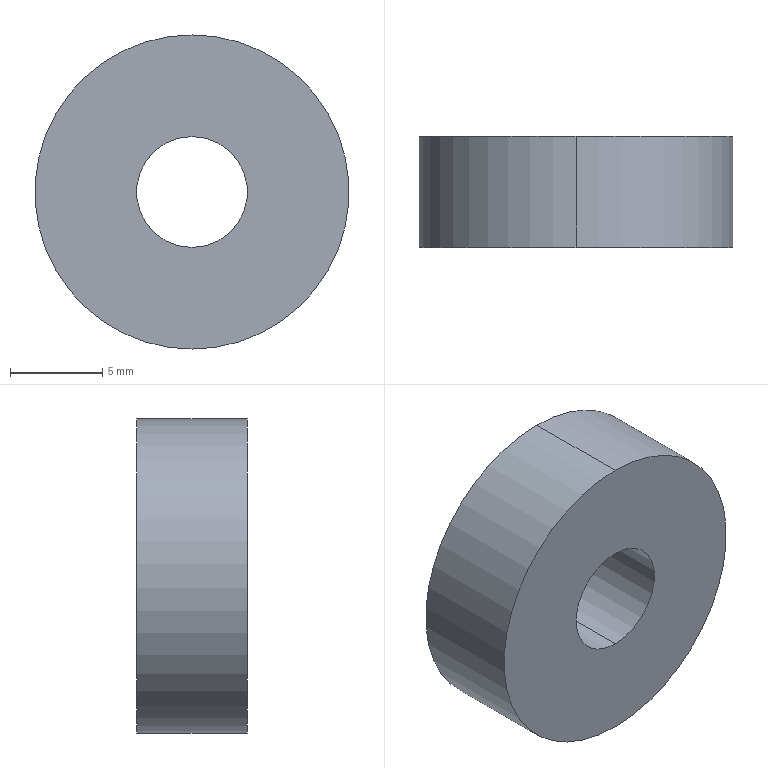Part | SolidWorks | features Extrusion 1 | 1 solid | 6 faces | box 17 x 6 x 17 mm | volume 1192 mm3 | cylinder 4 | plane 2 | commonest cylinder face diameters 6 x2 17 x2
STEP:
#1=CARTESIAN_POINT('',(0.,6.,-3.));
#2=VERTEX_POINT('',#1);
#3=CARTESIAN_POINT('',(0.,6.,3.));
#4=VERTEX_POINT('',#3);
#5=CARTESIAN_POINT('',(0.,6.,0.));
#6=DIRECTION('',(0.,1.,0.));
#7=DIRECTION('',(0.,0.,1.));
#8=AXIS2_PLACEMENT_3D('',#5,#6,#7);
#9=CIRCLE('',#8,3.);
#10=EDGE_CURVE('',#2,#4,#9,.T.);
#11=ORIENTED_EDGE('',*,*,#10,.T.);
#12=CARTESIAN_POINT('',(0.,0.,3.));
#13=VERTEX_POINT('',#12);
#14=CARTESIAN_POINT('',(0.,6.,3.));
#15=DIRECTION('',(0.,-1.,0.));
#16=VECTOR('',#15,1000.);
#17=LINE('',#14,#16);
#18=EDGE_CURVE('',#4,#13,#17,.T.);
#19=ORIENTED_EDGE('',*,*,#18,.T.);
#20=CARTESIAN_POINT('',(0.,0.,-3.));
#21=VERTEX_POINT('',#20);
#22=CARTESIAN_POINT('',(0.,0.,0.));
#23=DIRECTION('',(0.,1.,0.));
#24=DIRECTION('',(0.,0.,1.));
#25=AXIS2_PLACEMENT_3D('',#22,#23,#24);
#26=CIRCLE('',#25,3.);
#27=EDGE_CURVE('',#21,#13,#26,.T.);
#28=ORIENTED_EDGE('',*,*,#27,.F.);
#29=CARTESIAN_POINT('',(0.,6.,-3.));
#30=DIRECTION('',(0.,-1.,0.));
#31=VECTOR('',#30,1000.);
#32=LINE('',#29,#31);
#33=EDGE_CURVE('',#2,#21,#32,.T.);
#34=ORIENTED_EDGE('',*,*,#33,.F.);
#35=EDGE_LOOP('',(#11,#19,#28,#34));
#36=FACE_OUTER_BOUND('',#35,.T.);
#37=CARTESIAN_POINT('',(0.,6.,0.));
#38=DIRECTION('',(0.,-1.,0.));
#39=DIRECTION('',(0.,0.,-1.));
#40=AXIS2_PLACEMENT_3D('',#37,#38,#39);
#41=CYLINDRICAL_SURFACE('',#40,3.);
#42=ADVANCED_FACE('',(#36),#41,.F.);
#43=CARTESIAN_POINT('',(0.,6.,8.5));
#44=VERTEX_POINT('',#43);
#45=CARTESIAN_POINT('',(0.,6.,-8.5));
#46=VERTEX_POINT('',#45);
#47=CARTESIAN_POINT('',(0.,6.,0.));
#48=DIRECTION('',(0.,1.,0.));
#49=DIRECTION('',(0.,0.,1.));
#50=AXIS2_PLACEMENT_3D('',#47,#48,#49);
#51=CIRCLE('',#50,8.5);
#52=EDGE_CURVE('',#44,#46,#51,.T.);
#53=ORIENTED_EDGE('',*,*,#52,.F.);
#54=CARTESIAN_POINT('',(0.,0.,8.5));
#55=VERTEX_POINT('',#54);
#56=CARTESIAN_POINT('',(0.,6.,8.5));
#57=DIRECTION('',(0.,-1.,0.));
#58=VECTOR('',#57,1000.);
#59=LINE('',#56,#58);
#60=EDGE_CURVE('',#44,#55,#59,.T.);
#61=ORIENTED_EDGE('',*,*,#60,.T.);
#62=CARTESIAN_POINT('',(0.,0.,-8.5));
#63=VERTEX_POINT('',#62);
#64=CARTESIAN_POINT('',(0.,0.,0.));
#65=DIRECTION('',(0.,1.,0.));
#66=DIRECTION('',(0.,0.,1.));
#67=AXIS2_PLACEMENT_3D('',#64,#65,#66);
#68=CIRCLE('',#67,8.5);
#69=EDGE_CURVE('',#55,#63,#68,.T.);
#70=ORIENTED_EDGE('',*,*,#69,.T.);
#71=CARTESIAN_POINT('',(0.,6.,-8.5));
#72=DIRECTION('',(0.,-1.,0.));
#73=VECTOR('',#72,1000.);
#74=LINE('',#71,#73);
#75=EDGE_CURVE('',#46,#63,#74,.T.);
#76=ORIENTED_EDGE('',*,*,#75,.F.);
#77=EDGE_LOOP('',(#53,#61,#70,#76));
#78=FACE_OUTER_BOUND('',#77,.T.);
#79=CARTESIAN_POINT('',(0.,6.,0.));
#80=DIRECTION('',(0.,-1.,0.));
#81=DIRECTION('',(0.,0.,-1.));
#82=AXIS2_PLACEMENT_3D('',#79,#80,#81);
#83=CYLINDRICAL_SURFACE('',#82,8.5);
#84=ADVANCED_FACE('',(#78),#83,.T.);
#85=CARTESIAN_POINT('',(0.,6.,0.));
#86=DIRECTION('',(0.,1.,0.));
#87=DIRECTION('',(0.,0.,1.));
#88=AXIS2_PLACEMENT_3D('',#85,#86,#87);
#89=CIRCLE('',#88,8.5);
#90=EDGE_CURVE('',#46,#44,#89,.T.);
#91=ORIENTED_EDGE('',*,*,#90,.T.);
#92=ORIENTED_EDGE('',*,*,#52,.T.);
#93=EDGE_LOOP('',(#91,#92));
#94=FACE_OUTER_BOUND('',#93,.T.);
#95=ORIENTED_EDGE('',*,*,#10,.F.);
#96=CARTESIAN_POINT('',(0.,6.,0.));
#97=DIRECTION('',(0.,1.,0.));
#98=DIRECTION('',(0.,0.,1.));
#99=AXIS2_PLACEMENT_3D('',#96,#97,#98);
#100=CIRCLE('',#99,3.);
#101=EDGE_CURVE('',#4,#2,#100,.T.);
#102=ORIENTED_EDGE('',*,*,#101,.F.);
#103=EDGE_LOOP('',(#95,#102));
#104=FACE_BOUND('',#103,.T.);
#105=CARTESIAN_POINT('',(0.,6.,0.));
#106=DIRECTION('',(0.,1.,0.));
#107=DIRECTION('',(0.,0.,1.));
#108=AXIS2_PLACEMENT_3D('',#105,#106,#107);
#109=PLANE('',#108);
#110=ADVANCED_FACE('',(#94,#104),#109,.T.);
#111=CARTESIAN_POINT('',(0.,0.,0.));
#112=DIRECTION('',(0.,1.,0.));
#113=DIRECTION('',(0.,0.,1.));
#114=AXIS2_PLACEMENT_3D('',#111,#112,#113);
#115=CIRCLE('',#114,8.5);
#116=EDGE_CURVE('',#63,#55,#115,.T.);
#117=ORIENTED_EDGE('',*,*,#116,.F.);
#118=ORIENTED_EDGE('',*,*,#69,.F.);
#119=EDGE_LOOP('',(#117,#118));
#120=FACE_OUTER_BOUND('',#119,.T.);
#121=ORIENTED_EDGE('',*,*,#27,.T.);
#122=CARTESIAN_POINT('',(0.,0.,0.));
#123=DIRECTION('',(0.,1.,0.));
#124=DIRECTION('',(0.,0.,1.));
#125=AXIS2_PLACEMENT_3D('',#122,#123,#124);
#126=CIRCLE('',#125,3.);
#127=EDGE_CURVE('',#13,#21,#126,.T.);
#128=ORIENTED_EDGE('',*,*,#127,.T.);
#129=EDGE_LOOP('',(#121,#128));
#130=FACE_BOUND('',#129,.T.);
#131=CARTESIAN_POINT('',(0.,0.,0.));
#132=DIRECTION('',(0.,1.,0.));
#133=DIRECTION('',(0.,0.,1.));
#134=AXIS2_PLACEMENT_3D('',#131,#132,#133);
#135=PLANE('',#134);
#136=ADVANCED_FACE('',(#120,#130),#135,.F.);
#137=ORIENTED_EDGE('',*,*,#60,.F.);
#138=ORIENTED_EDGE('',*,*,#90,.F.);
#139=ORIENTED_EDGE('',*,*,#75,.T.);
#140=ORIENTED_EDGE('',*,*,#116,.T.);
#141=EDGE_LOOP('',(#137,#138,#139,#140));
#142=FACE_OUTER_BOUND('',#141,.T.);
#143=CARTESIAN_POINT('',(0.,6.,0.));
#144=DIRECTION('',(0.,-1.,0.));
#145=DIRECTION('',(0.,0.,-1.));
#146=AXIS2_PLACEMENT_3D('',#143,#144,#145);
#147=CYLINDRICAL_SURFACE('',#146,8.5);
#148=ADVANCED_FACE('',(#142),#147,.T.);
#149=ORIENTED_EDGE('',*,*,#18,.F.);
#150=ORIENTED_EDGE('',*,*,#101,.T.);
#151=ORIENTED_EDGE('',*,*,#33,.T.);
#152=ORIENTED_EDGE('',*,*,#127,.F.);
#153=EDGE_LOOP('',(#149,#150,#151,#152));
#154=FACE_OUTER_BOUND('',#153,.T.);
#155=CARTESIAN_POINT('',(0.,6.,0.));
#156=DIRECTION('',(0.,-1.,0.));
#157=DIRECTION('',(0.,0.,-1.));
#158=AXIS2_PLACEMENT_3D('',#155,#156,#157);
#159=CYLINDRICAL_SURFACE('',#158,3.);
#160=ADVANCED_FACE('',(#154),#159,.F.);
#161=CLOSED_SHELL('',(#42,#84,#110,#136,#148,#160));
#162=MANIFOLD_SOLID_BREP('',#161);
#163=CARTESIAN_POINT('',(0.,0.,0.));
#164=DIRECTION('',(0.,0.,1.));
#165=DIRECTION('',(1.,0.,0.));
#166=AXIS2_PLACEMENT_3D('',#163,#164,#165);
#167=(LENGTH_UNIT()NAMED_UNIT(*)SI_UNIT(.MILLI.,.METRE.));
#168=UNCERTAINTY_MEASURE_WITH_UNIT(LENGTH_MEASURE(0.00001),#167,'','');
#169=(NAMED_UNIT(*)PLANE_ANGLE_UNIT()SI_UNIT($,.RADIAN.));
#170=(NAMED_UNIT(*)SI_UNIT($,.STERADIAN.)SOLID_ANGLE_UNIT());
#171=(GEOMETRIC_REPRESENTATION_CONTEXT(3)GLOBAL_UNCERTAINTY_ASSIGNED_CONTEXT((#168))GLOBAL_UNIT_ASSIGNED_CONTEXT((#167,#169,#170))REPRESENTATION_CONTEXT('',''));
#172=ADVANCED_BREP_SHAPE_REPRESENTATION('',(#162,#166),#171);